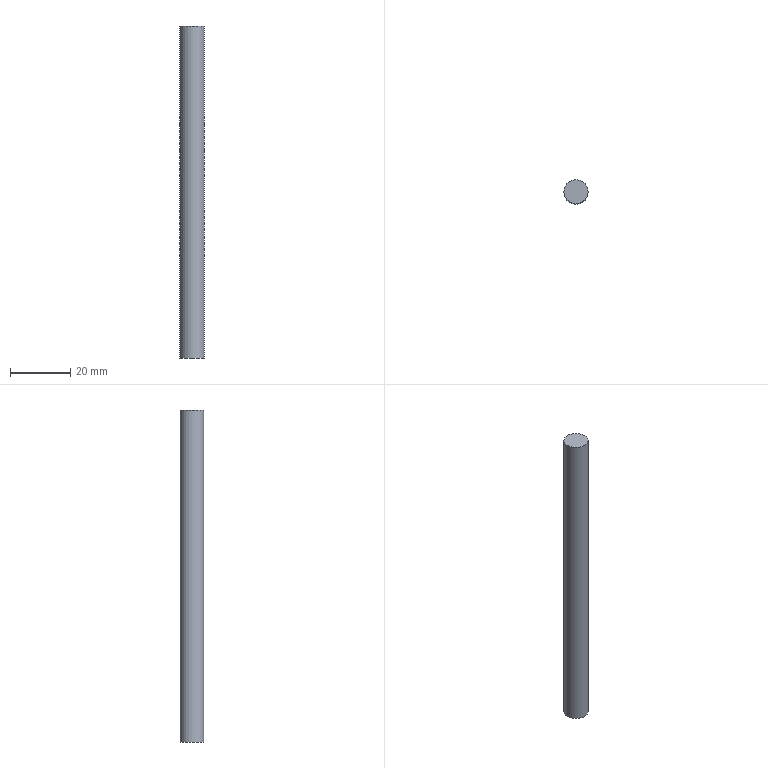Part | NX | features CYLINDER 1, DATUM_CSYS 1 | 1 solid | 3 faces | box 8 x 8 x 110 mm | volume 5529 mm3 | plane 2 | cylinder 1 | commonest cylinder face diameters 8 x1
STEP:
#1=CARTESIAN_POINT('',(4.,0.,110.));
#2=VERTEX_POINT('',#1);
#3=CARTESIAN_POINT('',(0.,0.,110.));
#4=DIRECTION('',(0.,0.,-1.));
#5=DIRECTION('',(1.,0.,0.));
#6=AXIS2_PLACEMENT_3D('',#3,#4,#5);
#7=CIRCLE('',#6,4.);
#8=EDGE_CURVE('',#2,#2,#7,.T.);
#9=ORIENTED_EDGE('',*,*,#8,.F.);
#10=EDGE_LOOP('',(#9));
#11=FACE_BOUND('',#10,.T.);
#12=CARTESIAN_POINT('',(0.,0.,110.));
#13=DIRECTION('',(0.,0.,1.));
#14=DIRECTION('',(1.,0.,0.));
#15=AXIS2_PLACEMENT_3D('',#12,#13,#14);
#16=PLANE('',#15);
#17=ADVANCED_FACE('',(#11),#16,.T.);
#18=CARTESIAN_POINT('',(4.,0.,0.));
#19=VERTEX_POINT('',#18);
#20=CARTESIAN_POINT('',(0.,0.,0.));
#21=DIRECTION('',(0.,0.,1.));
#22=DIRECTION('',(1.,0.,0.));
#23=AXIS2_PLACEMENT_3D('',#20,#21,#22);
#24=CIRCLE('',#23,4.);
#25=EDGE_CURVE('',#19,#19,#24,.T.);
#26=ORIENTED_EDGE('',*,*,#25,.F.);
#27=EDGE_LOOP('',(#26));
#28=FACE_BOUND('',#27,.T.);
#29=CARTESIAN_POINT('',(0.,0.,0.));
#30=DIRECTION('',(0.,0.,-1.));
#31=DIRECTION('',(-1.,0.,0.));
#32=AXIS2_PLACEMENT_3D('',#29,#30,#31);
#33=PLANE('',#32);
#34=ADVANCED_FACE('',(#28),#33,.T.);
#35=ORIENTED_EDGE('',*,*,#8,.T.);
#36=EDGE_LOOP('',(#35));
#37=FACE_BOUND('',#36,.T.);
#38=ORIENTED_EDGE('',*,*,#25,.T.);
#39=EDGE_LOOP('',(#38));
#40=FACE_BOUND('',#39,.T.);
#41=CARTESIAN_POINT('',(0.,0.,0.));
#42=DIRECTION('',(0.,0.,1.));
#43=DIRECTION('',(1.,0.,0.));
#44=AXIS2_PLACEMENT_3D('',#41,#42,#43);
#45=CYLINDRICAL_SURFACE('',#44,4.);
#46=ADVANCED_FACE('',(#37,#40),#45,.T.);
#47=CLOSED_SHELL('',(#17,#34,#46));
#48=MANIFOLD_SOLID_BREP('',#47);
#49=(LENGTH_UNIT()NAMED_UNIT(*)SI_UNIT(.MILLI.,.METRE.));
#50=UNCERTAINTY_MEASURE_WITH_UNIT(LENGTH_MEASURE(0.00001),#49,'','');
#51=(NAMED_UNIT(*)PLANE_ANGLE_UNIT()SI_UNIT($,.RADIAN.));
#52=(NAMED_UNIT(*)SI_UNIT($,.STERADIAN.)SOLID_ANGLE_UNIT());
#53=(GEOMETRIC_REPRESENTATION_CONTEXT(3)GLOBAL_UNCERTAINTY_ASSIGNED_CONTEXT((#50))GLOBAL_UNIT_ASSIGNED_CONTEXT((#49,#51,#52))REPRESENTATION_CONTEXT('',''));
#54=ADVANCED_BREP_SHAPE_REPRESENTATION('',(#48),#53);